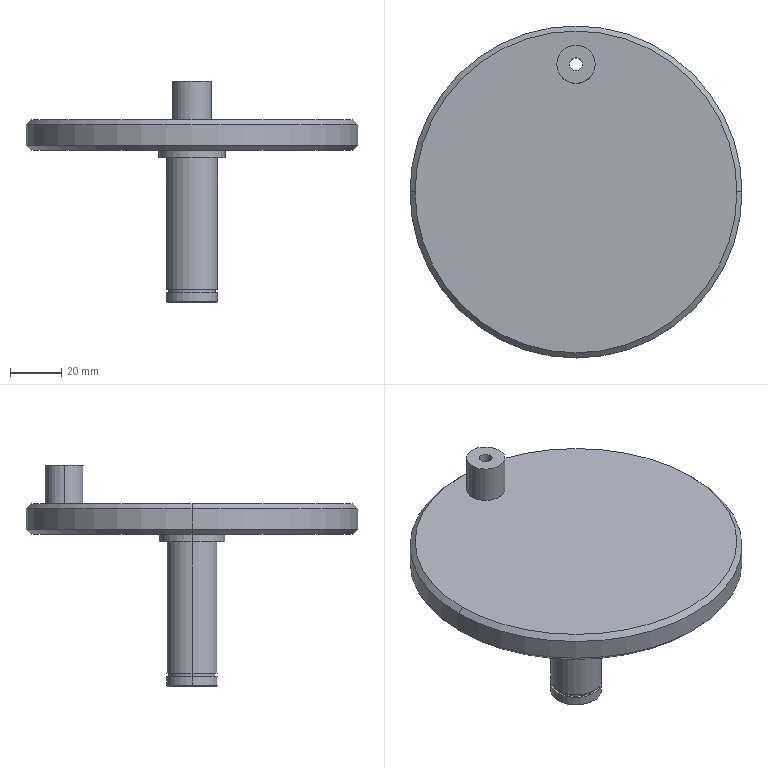Part | SolidWorks | features BaseBody 1 | 1 solid | 27 faces | box 130 x 130 x 86.7 mm | volume 179121 mm3 | cylinder 14 | plane 7 | cone 6 | commonest cylinder face diameters 20 x4 5 x2 15 x2 18.35 x2 26 x2 130 x2
STEP:
#1=CARTESIAN_POINT('',(-9.175,0.,-55.7));
#2=VERTEX_POINT('',#1);
#3=CARTESIAN_POINT('',(9.175,0.,-55.7));
#4=VERTEX_POINT('',#3);
#5=CARTESIAN_POINT('',(0.,0.,-55.7));
#6=DIRECTION('',(0.,0.,-1.));
#7=DIRECTION('',(1.,0.,0.));
#8=AXIS2_PLACEMENT_3D('',#5,#6,#7);
#9=CIRCLE('',#8,9.175);
#10=EDGE_CURVE('',#2,#4,#9,.T.);
#11=ORIENTED_EDGE('',*,*,#10,.F.);
#12=CARTESIAN_POINT('',(-9.175,0.,-54.5));
#13=VERTEX_POINT('',#12);
#14=CARTESIAN_POINT('',(-9.175,0.,-55.1));
#15=DIRECTION('',(0.,0.,1.));
#16=VECTOR('',#15,1000.);
#17=LINE('',#14,#16);
#18=EDGE_CURVE('',#2,#13,#17,.T.);
#19=ORIENTED_EDGE('',*,*,#18,.T.);
#20=CARTESIAN_POINT('',(9.175,0.,-54.5));
#21=VERTEX_POINT('',#20);
#22=CARTESIAN_POINT('',(0.,0.,-54.5));
#23=DIRECTION('',(0.,0.,-1.));
#24=DIRECTION('',(1.,0.,0.));
#25=AXIS2_PLACEMENT_3D('',#22,#23,#24);
#26=CIRCLE('',#25,9.175);
#27=EDGE_CURVE('',#13,#21,#26,.T.);
#28=ORIENTED_EDGE('',*,*,#27,.T.);
#29=CARTESIAN_POINT('',(9.175,0.,-55.1));
#30=DIRECTION('',(0.,0.,1.));
#31=VECTOR('',#30,1000.);
#32=LINE('',#29,#31);
#33=EDGE_CURVE('',#4,#21,#32,.T.);
#34=ORIENTED_EDGE('',*,*,#33,.F.);
#35=EDGE_LOOP('',(#11,#19,#28,#34));
#36=FACE_OUTER_BOUND('',#35,.T.);
#37=CARTESIAN_POINT('',(0.,0.,-55.1));
#38=DIRECTION('',(0.,0.,1.));
#39=DIRECTION('',(1.,0.,0.));
#40=AXIS2_PLACEMENT_3D('',#37,#38,#39);
#41=CYLINDRICAL_SURFACE('',#40,9.175);
#42=ADVANCED_FACE('',(#36),#41,.T.);
#43=CARTESIAN_POINT('',(10.,0.,-54.5));
#44=VERTEX_POINT('',#43);
#45=CARTESIAN_POINT('',(-10.,0.,-54.5));
#46=VERTEX_POINT('',#45);
#47=CARTESIAN_POINT('',(0.,0.,-54.5));
#48=DIRECTION('',(0.,0.,1.));
#49=DIRECTION('',(1.,0.,0.));
#50=AXIS2_PLACEMENT_3D('',#47,#48,#49);
#51=CIRCLE('',#50,10.);
#52=EDGE_CURVE('',#44,#46,#51,.T.);
#53=ORIENTED_EDGE('',*,*,#52,.T.);
#54=CARTESIAN_POINT('',(-10.,0.,-3.));
#55=VERTEX_POINT('',#54);
#56=CARTESIAN_POINT('',(-10.,0.,0.));
#57=DIRECTION('',(0.,0.,1.));
#58=VECTOR('',#57,1000.);
#59=LINE('',#56,#58);
#60=EDGE_CURVE('',#46,#55,#59,.T.);
#61=ORIENTED_EDGE('',*,*,#60,.T.);
#62=CARTESIAN_POINT('',(10.,0.,-3.));
#63=VERTEX_POINT('',#62);
#64=CARTESIAN_POINT('',(0.,0.,-3.));
#65=DIRECTION('',(0.,0.,-1.));
#66=DIRECTION('',(1.,0.,0.));
#67=AXIS2_PLACEMENT_3D('',#64,#65,#66);
#68=CIRCLE('',#67,10.);
#69=EDGE_CURVE('',#55,#63,#68,.T.);
#70=ORIENTED_EDGE('',*,*,#69,.T.);
#71=CARTESIAN_POINT('',(10.,0.,0.));
#72=DIRECTION('',(0.,0.,1.));
#73=VECTOR('',#72,1000.);
#74=LINE('',#71,#73);
#75=EDGE_CURVE('',#44,#63,#74,.T.);
#76=ORIENTED_EDGE('',*,*,#75,.F.);
#77=EDGE_LOOP('',(#53,#61,#70,#76));
#78=FACE_OUTER_BOUND('',#77,.T.);
#79=CARTESIAN_POINT('',(0.,0.,0.));
#80=DIRECTION('',(0.,0.,1.));
#81=DIRECTION('',(1.,0.,0.));
#82=AXIS2_PLACEMENT_3D('',#79,#80,#81);
#83=CYLINDRICAL_SURFACE('',#82,10.);
#84=ADVANCED_FACE('',(#78),#83,.T.);
#85=CARTESIAN_POINT('',(9.5,0.,-59.7));
#86=VERTEX_POINT('',#85);
#87=CARTESIAN_POINT('',(-9.5,0.,-59.7));
#88=VERTEX_POINT('',#87);
#89=CARTESIAN_POINT('',(0.,0.,-59.7));
#90=DIRECTION('',(0.,0.,1.));
#91=DIRECTION('',(1.,0.,0.));
#92=AXIS2_PLACEMENT_3D('',#89,#90,#91);
#93=CIRCLE('',#92,9.5);
#94=EDGE_CURVE('',#86,#88,#93,.T.);
#95=ORIENTED_EDGE('',*,*,#94,.T.);
#96=CARTESIAN_POINT('',(-10.,0.,-59.2));
#97=VERTEX_POINT('',#96);
#98=CARTESIAN_POINT('',(-9.75,0.,-59.45));
#99=DIRECTION('',(-0.7071,0.,0.7071));
#100=VECTOR('',#99,1000.);
#101=LINE('',#98,#100);
#102=EDGE_CURVE('',#88,#97,#101,.T.);
#103=ORIENTED_EDGE('',*,*,#102,.T.);
#104=CARTESIAN_POINT('',(10.,0.,-59.2));
#105=VERTEX_POINT('',#104);
#106=CARTESIAN_POINT('',(0.,0.,-59.2));
#107=DIRECTION('',(0.,0.,-1.));
#108=DIRECTION('',(1.,0.,0.));
#109=AXIS2_PLACEMENT_3D('',#106,#107,#108);
#110=CIRCLE('',#109,10.);
#111=EDGE_CURVE('',#97,#105,#110,.T.);
#112=ORIENTED_EDGE('',*,*,#111,.T.);
#113=CARTESIAN_POINT('',(9.75,0.,-59.45));
#114=DIRECTION('',(0.7071,0.,0.7071));
#115=VECTOR('',#114,1000.);
#116=LINE('',#113,#115);
#117=EDGE_CURVE('',#86,#105,#116,.T.);
#118=ORIENTED_EDGE('',*,*,#117,.F.);
#119=EDGE_LOOP('',(#95,#103,#112,#118));
#120=FACE_OUTER_BOUND('',#119,.T.);
#121=CARTESIAN_POINT('',(0.,0.,-59.45));
#122=DIRECTION('',(0.,0.,1.));
#123=DIRECTION('',(1.,0.,0.));
#124=AXIS2_PLACEMENT_3D('',#121,#122,#123);
#125=CONICAL_SURFACE('',#124,9.75,0.7854);
#126=ADVANCED_FACE('',(#120),#125,.T.);
#127=ORIENTED_EDGE('',*,*,#111,.F.);
#128=CARTESIAN_POINT('',(-10.,0.,-55.7));
#129=VERTEX_POINT('',#128);
#130=CARTESIAN_POINT('',(-10.,0.,0.));
#131=DIRECTION('',(0.,0.,1.));
#132=VECTOR('',#131,1000.);
#133=LINE('',#130,#132);
#134=EDGE_CURVE('',#97,#129,#133,.T.);
#135=ORIENTED_EDGE('',*,*,#134,.T.);
#136=CARTESIAN_POINT('',(10.,0.,-55.7));
#137=VERTEX_POINT('',#136);
#138=CARTESIAN_POINT('',(0.,0.,-55.7));
#139=DIRECTION('',(0.,0.,-1.));
#140=DIRECTION('',(1.,0.,0.));
#141=AXIS2_PLACEMENT_3D('',#138,#139,#140);
#142=CIRCLE('',#141,10.);
#143=EDGE_CURVE('',#129,#137,#142,.T.);
#144=ORIENTED_EDGE('',*,*,#143,.T.);
#145=CARTESIAN_POINT('',(10.,0.,0.));
#146=DIRECTION('',(0.,0.,1.));
#147=VECTOR('',#146,1000.);
#148=LINE('',#145,#147);
#149=EDGE_CURVE('',#105,#137,#148,.T.);
#150=ORIENTED_EDGE('',*,*,#149,.F.);
#151=EDGE_LOOP('',(#127,#135,#144,#150));
#152=FACE_OUTER_BOUND('',#151,.T.);
#153=CARTESIAN_POINT('',(0.,0.,0.));
#154=DIRECTION('',(0.,0.,1.));
#155=DIRECTION('',(1.,0.,0.));
#156=AXIS2_PLACEMENT_3D('',#153,#154,#155);
#157=CYLINDRICAL_SURFACE('',#156,10.);
#158=ADVANCED_FACE('',(#152),#157,.T.);
#159=CARTESIAN_POINT('',(-63.,0.,12.));
#160=VERTEX_POINT('',#159);
#161=CARTESIAN_POINT('',(63.,0.,12.));
#162=VERTEX_POINT('',#161);
#163=CARTESIAN_POINT('',(0.,0.,12.));
#164=DIRECTION('',(0.,0.,-1.));
#165=DIRECTION('',(-1.,0.,0.));
#166=AXIS2_PLACEMENT_3D('',#163,#164,#165);
#167=CIRCLE('',#166,63.);
#168=EDGE_CURVE('',#160,#162,#167,.T.);
#169=ORIENTED_EDGE('',*,*,#168,.T.);
#170=CARTESIAN_POINT('',(65.,0.,10.));
#171=VERTEX_POINT('',#170);
#172=CARTESIAN_POINT('',(64.,0.,11.));
#173=DIRECTION('',(0.7071,0.,-0.7071));
#174=VECTOR('',#173,1000.);
#175=LINE('',#172,#174);
#176=EDGE_CURVE('',#162,#171,#175,.T.);
#177=ORIENTED_EDGE('',*,*,#176,.T.);
#178=CARTESIAN_POINT('',(-65.,0.,10.));
#179=VERTEX_POINT('',#178);
#180=CARTESIAN_POINT('',(0.,0.,10.));
#181=DIRECTION('',(0.,0.,1.));
#182=DIRECTION('',(-1.,0.,0.));
#183=AXIS2_PLACEMENT_3D('',#180,#181,#182);
#184=CIRCLE('',#183,65.);
#185=EDGE_CURVE('',#171,#179,#184,.T.);
#186=ORIENTED_EDGE('',*,*,#185,.T.);
#187=CARTESIAN_POINT('',(-64.,0.,11.));
#188=DIRECTION('',(-0.7071,0.,-0.7071));
#189=VECTOR('',#188,1000.);
#190=LINE('',#187,#189);
#191=EDGE_CURVE('',#160,#179,#190,.T.);
#192=ORIENTED_EDGE('',*,*,#191,.F.);
#193=EDGE_LOOP('',(#169,#177,#186,#192));
#194=FACE_OUTER_BOUND('',#193,.T.);
#195=CARTESIAN_POINT('',(0.,0.,11.));
#196=DIRECTION('',(0.,0.,-1.));
#197=DIRECTION('',(-1.,0.,0.));
#198=AXIS2_PLACEMENT_3D('',#195,#196,#197);
#199=CONICAL_SURFACE('',#198,64.,0.7854);
#200=ADVANCED_FACE('',(#194),#199,.T.);
#201=ORIENTED_EDGE('',*,*,#185,.F.);
#202=CARTESIAN_POINT('',(65.,0.,2.));
#203=VERTEX_POINT('',#202);
#204=CARTESIAN_POINT('',(65.,0.,0.));
#205=DIRECTION('',(0.,0.,-1.));
#206=VECTOR('',#205,1000.);
#207=LINE('',#204,#206);
#208=EDGE_CURVE('',#171,#203,#207,.T.);
#209=ORIENTED_EDGE('',*,*,#208,.T.);
#210=CARTESIAN_POINT('',(-65.,0.,2.));
#211=VERTEX_POINT('',#210);
#212=CARTESIAN_POINT('',(0.,0.,2.));
#213=DIRECTION('',(0.,0.,-1.));
#214=DIRECTION('',(-1.,0.,0.));
#215=AXIS2_PLACEMENT_3D('',#212,#213,#214);
#216=CIRCLE('',#215,65.);
#217=EDGE_CURVE('',#211,#203,#216,.T.);
#218=ORIENTED_EDGE('',*,*,#217,.F.);
#219=CARTESIAN_POINT('',(-65.,0.,0.));
#220=DIRECTION('',(0.,0.,-1.));
#221=VECTOR('',#220,1000.);
#222=LINE('',#219,#221);
#223=EDGE_CURVE('',#179,#211,#222,.T.);
#224=ORIENTED_EDGE('',*,*,#223,.F.);
#225=EDGE_LOOP('',(#201,#209,#218,#224));
#226=FACE_OUTER_BOUND('',#225,.T.);
#227=CARTESIAN_POINT('',(0.,0.,0.));
#228=DIRECTION('',(0.,0.,-1.));
#229=DIRECTION('',(-1.,0.,0.));
#230=AXIS2_PLACEMENT_3D('',#227,#228,#229);
#231=CYLINDRICAL_SURFACE('',#230,65.);
#232=ADVANCED_FACE('',(#226),#231,.T.);
#233=CARTESIAN_POINT('',(-63.,0.,0.));
#234=VERTEX_POINT('',#233);
#235=CARTESIAN_POINT('',(63.,0.,0.));
#236=VERTEX_POINT('',#235);
#237=CARTESIAN_POINT('',(0.,0.,0.));
#238=DIRECTION('',(0.,0.,1.));
#239=DIRECTION('',(-1.,0.,0.));
#240=AXIS2_PLACEMENT_3D('',#237,#238,#239);
#241=CIRCLE('',#240,63.);
#242=EDGE_CURVE('',#234,#236,#241,.T.);
#243=ORIENTED_EDGE('',*,*,#242,.T.);
#244=CARTESIAN_POINT('',(64.,0.,1.));
#245=DIRECTION('',(0.7071,0.,0.7071));
#246=VECTOR('',#245,1000.);
#247=LINE('',#244,#246);
#248=EDGE_CURVE('',#236,#203,#247,.T.);
#249=ORIENTED_EDGE('',*,*,#248,.T.);
#250=CARTESIAN_POINT('',(0.,0.,2.));
#251=DIRECTION('',(0.,0.,-1.));
#252=DIRECTION('',(-1.,0.,0.));
#253=AXIS2_PLACEMENT_3D('',#250,#251,#252);
#254=CIRCLE('',#253,65.);
#255=EDGE_CURVE('',#203,#211,#254,.T.);
#256=ORIENTED_EDGE('',*,*,#255,.T.);
#257=CARTESIAN_POINT('',(-64.,0.,1.));
#258=DIRECTION('',(-0.7071,0.,0.7071));
#259=VECTOR('',#258,1000.);
#260=LINE('',#257,#259);
#261=EDGE_CURVE('',#234,#211,#260,.T.);
#262=ORIENTED_EDGE('',*,*,#261,.F.);
#263=EDGE_LOOP('',(#243,#249,#256,#262));
#264=FACE_OUTER_BOUND('',#263,.T.);
#265=CARTESIAN_POINT('',(0.,0.,1.));
#266=DIRECTION('',(0.,0.,1.));
#267=DIRECTION('',(-1.,0.,0.));
#268=AXIS2_PLACEMENT_3D('',#265,#266,#267);
#269=CONICAL_SURFACE('',#268,64.,0.7854);
#270=ADVANCED_FACE('',(#264),#269,.T.);
#271=CARTESIAN_POINT('',(-13.,0.,-3.));
#272=VERTEX_POINT('',#271);
#273=CARTESIAN_POINT('',(13.,0.,-3.));
#274=VERTEX_POINT('',#273);
#275=CARTESIAN_POINT('',(0.,0.,-3.));
#276=DIRECTION('',(0.,0.,-1.));
#277=DIRECTION('',(1.,0.,0.));
#278=AXIS2_PLACEMENT_3D('',#275,#276,#277);
#279=CIRCLE('',#278,13.);
#280=EDGE_CURVE('',#272,#274,#279,.T.);
#281=ORIENTED_EDGE('',*,*,#280,.F.);
#282=CARTESIAN_POINT('',(-13.,0.,0.));
#283=VERTEX_POINT('',#282);
#284=CARTESIAN_POINT('',(-13.,0.,0.));
#285=DIRECTION('',(0.,0.,1.));
#286=VECTOR('',#285,1000.);
#287=LINE('',#284,#286);
#288=EDGE_CURVE('',#272,#283,#287,.T.);
#289=ORIENTED_EDGE('',*,*,#288,.T.);
#290=CARTESIAN_POINT('',(13.,0.,0.));
#291=VERTEX_POINT('',#290);
#292=CARTESIAN_POINT('',(0.,0.,0.));
#293=DIRECTION('',(0.,0.,1.));
#294=DIRECTION('',(1.,0.,0.));
#295=AXIS2_PLACEMENT_3D('',#292,#293,#294);
#296=CIRCLE('',#295,13.);
#297=EDGE_CURVE('',#291,#283,#296,.T.);
#298=ORIENTED_EDGE('',*,*,#297,.F.);
#299=CARTESIAN_POINT('',(13.,0.,0.));
#300=DIRECTION('',(0.,0.,1.));
#301=VECTOR('',#300,1000.);
#302=LINE('',#299,#301);
#303=EDGE_CURVE('',#274,#291,#302,.T.);
#304=ORIENTED_EDGE('',*,*,#303,.F.);
#305=EDGE_LOOP('',(#281,#289,#298,#304));
#306=FACE_OUTER_BOUND('',#305,.T.);
#307=CARTESIAN_POINT('',(0.,0.,0.));
#308=DIRECTION('',(0.,0.,1.));
#309=DIRECTION('',(1.,0.,0.));
#310=AXIS2_PLACEMENT_3D('',#307,#308,#309);
#311=CYLINDRICAL_SURFACE('',#310,13.);
#312=ADVANCED_FACE('',(#306),#311,.T.);
#313=CARTESIAN_POINT('',(2.5,50.,0.));
#314=VERTEX_POINT('',#313);
#315=CARTESIAN_POINT('',(-2.5,50.,0.));
#316=VERTEX_POINT('',#315);
#317=CARTESIAN_POINT('',(0.,50.,0.));
#318=DIRECTION('',(0.,0.,1.));
#319=DIRECTION('',(-1.,0.,0.));
#320=AXIS2_PLACEMENT_3D('',#317,#318,#319);
#321=CIRCLE('',#320,2.5);
#322=EDGE_CURVE('',#314,#316,#321,.T.);
#323=ORIENTED_EDGE('',*,*,#322,.F.);
#324=CARTESIAN_POINT('',(2.5,50.,27.));
#325=VERTEX_POINT('',#324);
#326=CARTESIAN_POINT('',(2.5,50.,27.));
#327=DIRECTION('',(0.,0.,1.));
#328=VECTOR('',#327,1000.);
#329=LINE('',#326,#328);
#330=EDGE_CURVE('',#314,#325,#329,.T.);
#331=ORIENTED_EDGE('',*,*,#330,.T.);
#332=CARTESIAN_POINT('',(-2.5,50.,27.));
#333=VERTEX_POINT('',#332);
#334=CARTESIAN_POINT('',(0.,50.,27.));
#335=DIRECTION('',(0.,0.,-1.));
#336=DIRECTION('',(-1.,0.,0.));
#337=AXIS2_PLACEMENT_3D('',#334,#335,#336);
#338=CIRCLE('',#337,2.5);
#339=EDGE_CURVE('',#333,#325,#338,.T.);
#340=ORIENTED_EDGE('',*,*,#339,.F.);
#341=CARTESIAN_POINT('',(-2.5,50.,27.));
#342=DIRECTION('',(0.,0.,1.));
#343=VECTOR('',#342,1000.);
#344=LINE('',#341,#343);
#345=EDGE_CURVE('',#316,#333,#344,.T.);
#346=ORIENTED_EDGE('',*,*,#345,.F.);
#347=EDGE_LOOP('',(#323,#331,#340,#346));
#348=FACE_OUTER_BOUND('',#347,.T.);
#349=CARTESIAN_POINT('',(0.,50.,27.));
#350=DIRECTION('',(0.,0.,1.));
#351=DIRECTION('',(-1.,0.,0.));
#352=AXIS2_PLACEMENT_3D('',#349,#350,#351);
#353=CYLINDRICAL_SURFACE('',#352,2.5);
#354=ADVANCED_FACE('',(#348),#353,.F.);
#355=CARTESIAN_POINT('',(7.5,50.,27.));
#356=VERTEX_POINT('',#355);
#357=CARTESIAN_POINT('',(-7.5,50.,27.));
#358=VERTEX_POINT('',#357);
#359=CARTESIAN_POINT('',(0.,50.,27.));
#360=DIRECTION('',(0.,0.,1.));
#361=DIRECTION('',(-1.,0.,0.));
#362=AXIS2_PLACEMENT_3D('',#359,#360,#361);
#363=CIRCLE('',#362,7.5);
#364=EDGE_CURVE('',#356,#358,#363,.T.);
#365=ORIENTED_EDGE('',*,*,#364,.F.);
#366=CARTESIAN_POINT('',(7.5,50.,12.));
#367=VERTEX_POINT('',#366);
#368=CARTESIAN_POINT('',(7.5,50.,12.));
#369=DIRECTION('',(0.,0.,-1.));
#370=VECTOR('',#369,1000.);
#371=LINE('',#368,#370);
#372=EDGE_CURVE('',#356,#367,#371,.T.);
#373=ORIENTED_EDGE('',*,*,#372,.T.);
#374=CARTESIAN_POINT('',(-7.5,50.,12.));
#375=VERTEX_POINT('',#374);
#376=CARTESIAN_POINT('',(0.,50.,12.));
#377=DIRECTION('',(0.,0.,-1.));
#378=DIRECTION('',(-1.,0.,0.));
#379=AXIS2_PLACEMENT_3D('',#376,#377,#378);
#380=CIRCLE('',#379,7.5);
#381=EDGE_CURVE('',#375,#367,#380,.T.);
#382=ORIENTED_EDGE('',*,*,#381,.F.);
#383=CARTESIAN_POINT('',(-7.5,50.,12.));
#384=DIRECTION('',(0.,0.,-1.));
#385=VECTOR('',#384,1000.);
#386=LINE('',#383,#385);
#387=EDGE_CURVE('',#358,#375,#386,.T.);
#388=ORIENTED_EDGE('',*,*,#387,.F.);
#389=EDGE_LOOP('',(#365,#373,#382,#388));
#390=FACE_OUTER_BOUND('',#389,.T.);
#391=CARTESIAN_POINT('',(0.,50.,12.));
#392=DIRECTION('',(0.,0.,-1.));
#393=DIRECTION('',(-1.,0.,0.));
#394=AXIS2_PLACEMENT_3D('',#391,#392,#393);
#395=CYLINDRICAL_SURFACE('',#394,7.5);
#396=ADVANCED_FACE('',(#390),#395,.T.);
#397=CARTESIAN_POINT('',(0.,0.,-55.7));
#398=DIRECTION('',(0.,0.,-1.));
#399=DIRECTION('',(1.,0.,0.));
#400=AXIS2_PLACEMENT_3D('',#397,#398,#399);
#401=CIRCLE('',#400,9.175);
#402=EDGE_CURVE('',#4,#2,#401,.T.);
#403=ORIENTED_EDGE('',*,*,#402,.T.);
#404=ORIENTED_EDGE('',*,*,#10,.T.);
#405=EDGE_LOOP('',(#403,#404));
#406=FACE_BOUND('',#405,.T.);
#407=CARTESIAN_POINT('',(0.,0.,-55.7));
#408=DIRECTION('',(0.,0.,-1.));
#409=DIRECTION('',(1.,0.,0.));
#410=AXIS2_PLACEMENT_3D('',#407,#408,#409);
#411=CIRCLE('',#410,10.);
#412=EDGE_CURVE('',#137,#129,#411,.T.);
#413=ORIENTED_EDGE('',*,*,#412,.F.);
#414=ORIENTED_EDGE('',*,*,#143,.F.);
#415=EDGE_LOOP('',(#413,#414));
#416=FACE_OUTER_BOUND('',#415,.T.);
#417=CARTESIAN_POINT('',(9.175,0.,-55.7));
#418=DIRECTION('',(0.,0.,-1.));
#419=DIRECTION('',(0.,-1.,0.));
#420=AXIS2_PLACEMENT_3D('',#417,#418,#419);
#421=PLANE('',#420);
#422=ADVANCED_FACE('',(#406,#416),#421,.F.);
#423=CARTESIAN_POINT('',(0.,0.,-54.5));
#424=DIRECTION('',(0.,0.,-1.));
#425=DIRECTION('',(1.,0.,0.));
#426=AXIS2_PLACEMENT_3D('',#423,#424,#425);
#427=CIRCLE('',#426,9.175);
#428=EDGE_CURVE('',#21,#13,#427,.T.);
#429=ORIENTED_EDGE('',*,*,#428,.F.);
#430=ORIENTED_EDGE('',*,*,#27,.F.);
#431=EDGE_LOOP('',(#429,#430));
#432=FACE_BOUND('',#431,.T.);
#433=ORIENTED_EDGE('',*,*,#52,.F.);
#434=CARTESIAN_POINT('',(0.,0.,-54.5));
#435=DIRECTION('',(0.,0.,1.));
#436=DIRECTION('',(1.,0.,0.));
#437=AXIS2_PLACEMENT_3D('',#434,#435,#436);
#438=CIRCLE('',#437,10.);
#439=EDGE_CURVE('',#46,#44,#438,.T.);
#440=ORIENTED_EDGE('',*,*,#439,.F.);
#441=EDGE_LOOP('',(#433,#440));
#442=FACE_OUTER_BOUND('',#441,.T.);
#443=CARTESIAN_POINT('',(18.451,0.,-54.5));
#444=DIRECTION('',(0.,0.,1.));
#445=DIRECTION('',(1.,0.,0.));
#446=AXIS2_PLACEMENT_3D('',#443,#444,#445);
#447=PLANE('',#446);
#448=ADVANCED_FACE('',(#432,#442),#447,.F.);
#449=ORIENTED_EDGE('',*,*,#94,.F.);
#450=CARTESIAN_POINT('',(0.,0.,-59.7));
#451=DIRECTION('',(0.,0.,1.));
#452=DIRECTION('',(1.,0.,0.));
#453=AXIS2_PLACEMENT_3D('',#450,#451,#452);
#454=CIRCLE('',#453,9.5);
#455=EDGE_CURVE('',#88,#86,#454,.T.);
#456=ORIENTED_EDGE('',*,*,#455,.F.);
#457=EDGE_LOOP('',(#449,#456));
#458=FACE_OUTER_BOUND('',#457,.T.);
#459=CARTESIAN_POINT('',(0.,0.,-59.7));
#460=DIRECTION('',(0.,0.,1.));
#461=DIRECTION('',(1.,0.,0.));
#462=AXIS2_PLACEMENT_3D('',#459,#460,#461);
#463=PLANE('',#462);
#464=ADVANCED_FACE('',(#458),#463,.F.);
#465=ORIENTED_EDGE('',*,*,#381,.T.);
#466=CARTESIAN_POINT('',(0.,50.,12.));
#467=DIRECTION('',(0.,0.,-1.));
#468=DIRECTION('',(-1.,0.,0.));
#469=AXIS2_PLACEMENT_3D('',#466,#467,#468);
#470=CIRCLE('',#469,7.5);
#471=EDGE_CURVE('',#367,#375,#470,.T.);
#472=ORIENTED_EDGE('',*,*,#471,.T.);
#473=EDGE_LOOP('',(#465,#472));
#474=FACE_BOUND('',#473,.T.);
#475=ORIENTED_EDGE('',*,*,#168,.F.);
#476=CARTESIAN_POINT('',(0.,0.,12.));
#477=DIRECTION('',(0.,0.,-1.));
#478=DIRECTION('',(-1.,0.,0.));
#479=AXIS2_PLACEMENT_3D('',#476,#477,#478);
#480=CIRCLE('',#479,63.);
#481=EDGE_CURVE('',#162,#160,#480,.T.);
#482=ORIENTED_EDGE('',*,*,#481,.F.);
#483=EDGE_LOOP('',(#475,#482));
#484=FACE_OUTER_BOUND('',#483,.T.);
#485=CARTESIAN_POINT('',(0.,0.,12.));
#486=DIRECTION('',(0.,0.,1.));
#487=DIRECTION('',(1.,0.,0.));
#488=AXIS2_PLACEMENT_3D('',#485,#486,#487);
#489=PLANE('',#488);
#490=ADVANCED_FACE('',(#474,#484),#489,.T.);
#491=CARTESIAN_POINT('',(0.,50.,0.));
#492=DIRECTION('',(0.,0.,1.));
#493=DIRECTION('',(-1.,0.,0.));
#494=AXIS2_PLACEMENT_3D('',#491,#492,#493);
#495=CIRCLE('',#494,2.5);
#496=EDGE_CURVE('',#316,#314,#495,.T.);
#497=ORIENTED_EDGE('',*,*,#496,.T.);
#498=ORIENTED_EDGE('',*,*,#322,.T.);
#499=EDGE_LOOP('',(#497,#498));
#500=FACE_BOUND('',#499,.T.);
#501=ORIENTED_EDGE('',*,*,#297,.T.);
#502=CARTESIAN_POINT('',(0.,0.,0.));
#503=DIRECTION('',(0.,0.,1.));
#504=DIRECTION('',(1.,0.,0.));
#505=AXIS2_PLACEMENT_3D('',#502,#503,#504);
#506=CIRCLE('',#505,13.);
#507=EDGE_CURVE('',#283,#291,#506,.T.);
#508=ORIENTED_EDGE('',*,*,#507,.T.);
#509=EDGE_LOOP('',(#501,#508));
#510=FACE_BOUND('',#509,.T.);
#511=ORIENTED_EDGE('',*,*,#242,.F.);
#512=CARTESIAN_POINT('',(0.,0.,0.));
#513=DIRECTION('',(0.,0.,1.));
#514=DIRECTION('',(-1.,0.,0.));
#515=AXIS2_PLACEMENT_3D('',#512,#513,#514);
#516=CIRCLE('',#515,63.);
#517=EDGE_CURVE('',#236,#234,#516,.T.);
#518=ORIENTED_EDGE('',*,*,#517,.F.);
#519=EDGE_LOOP('',(#511,#518));
#520=FACE_OUTER_BOUND('',#519,.T.);
#521=CARTESIAN_POINT('',(0.,0.,0.));
#522=DIRECTION('',(0.,0.,1.));
#523=DIRECTION('',(1.,0.,0.));
#524=AXIS2_PLACEMENT_3D('',#521,#522,#523);
#525=PLANE('',#524);
#526=ADVANCED_FACE('',(#500,#510,#520),#525,.F.);
#527=CARTESIAN_POINT('',(0.,0.,-3.));
#528=DIRECTION('',(0.,0.,-1.));
#529=DIRECTION('',(1.,0.,0.));
#530=AXIS2_PLACEMENT_3D('',#527,#528,#529);
#531=CIRCLE('',#530,10.);
#532=EDGE_CURVE('',#63,#55,#531,.T.);
#533=ORIENTED_EDGE('',*,*,#532,.F.);
#534=ORIENTED_EDGE('',*,*,#69,.F.);
#535=EDGE_LOOP('',(#533,#534));
#536=FACE_BOUND('',#535,.T.);
#537=CARTESIAN_POINT('',(0.,0.,-3.));
#538=DIRECTION('',(0.,0.,-1.));
#539=DIRECTION('',(1.,0.,0.));
#540=AXIS2_PLACEMENT_3D('',#537,#538,#539);
#541=CIRCLE('',#540,13.);
#542=EDGE_CURVE('',#274,#272,#541,.T.);
#543=ORIENTED_EDGE('',*,*,#542,.T.);
#544=ORIENTED_EDGE('',*,*,#280,.T.);
#545=EDGE_LOOP('',(#543,#544));
#546=FACE_OUTER_BOUND('',#545,.T.);
#547=CARTESIAN_POINT('',(0.,0.,-3.));
#548=DIRECTION('',(0.,0.,1.));
#549=DIRECTION('',(1.,0.,0.));
#550=AXIS2_PLACEMENT_3D('',#547,#548,#549);
#551=PLANE('',#550);
#552=ADVANCED_FACE('',(#536,#546),#551,.F.);
#553=ORIENTED_EDGE('',*,*,#339,.T.);
#554=CARTESIAN_POINT('',(0.,50.,27.));
#555=DIRECTION('',(0.,0.,-1.));
#556=DIRECTION('',(-1.,0.,0.));
#557=AXIS2_PLACEMENT_3D('',#554,#555,#556);
#558=CIRCLE('',#557,2.5);
#559=EDGE_CURVE('',#325,#333,#558,.T.);
#560=ORIENTED_EDGE('',*,*,#559,.T.);
#561=EDGE_LOOP('',(#553,#560));
#562=FACE_BOUND('',#561,.T.);
#563=CARTESIAN_POINT('',(0.,50.,27.));
#564=DIRECTION('',(0.,0.,1.));
#565=DIRECTION('',(-1.,0.,0.));
#566=AXIS2_PLACEMENT_3D('',#563,#564,#565);
#567=CIRCLE('',#566,7.5);
#568=EDGE_CURVE('',#358,#356,#567,.T.);
#569=ORIENTED_EDGE('',*,*,#568,.T.);
#570=ORIENTED_EDGE('',*,*,#364,.T.);
#571=EDGE_LOOP('',(#569,#570));
#572=FACE_OUTER_BOUND('',#571,.T.);
#573=CARTESIAN_POINT('',(0.,50.,27.));
#574=DIRECTION('',(0.,0.,1.));
#575=DIRECTION('',(1.,0.,0.));
#576=AXIS2_PLACEMENT_3D('',#573,#574,#575);
#577=PLANE('',#576);
#578=ADVANCED_FACE('',(#562,#572),#577,.T.);
#579=ORIENTED_EDGE('',*,*,#372,.F.);
#580=ORIENTED_EDGE('',*,*,#568,.F.);
#581=ORIENTED_EDGE('',*,*,#387,.T.);
#582=ORIENTED_EDGE('',*,*,#471,.F.);
#583=EDGE_LOOP('',(#579,#580,#581,#582));
#584=FACE_OUTER_BOUND('',#583,.T.);
#585=CARTESIAN_POINT('',(0.,50.,12.));
#586=DIRECTION('',(0.,0.,-1.));
#587=DIRECTION('',(-1.,0.,0.));
#588=AXIS2_PLACEMENT_3D('',#585,#586,#587);
#589=CYLINDRICAL_SURFACE('',#588,7.5);
#590=ADVANCED_FACE('',(#584),#589,.T.);
#591=ORIENTED_EDGE('',*,*,#330,.F.);
#592=ORIENTED_EDGE('',*,*,#496,.F.);
#593=ORIENTED_EDGE('',*,*,#345,.T.);
#594=ORIENTED_EDGE('',*,*,#559,.F.);
#595=EDGE_LOOP('',(#591,#592,#593,#594));
#596=FACE_OUTER_BOUND('',#595,.T.);
#597=CARTESIAN_POINT('',(0.,50.,27.));
#598=DIRECTION('',(0.,0.,1.));
#599=DIRECTION('',(-1.,0.,0.));
#600=AXIS2_PLACEMENT_3D('',#597,#598,#599);
#601=CYLINDRICAL_SURFACE('',#600,2.5);
#602=ADVANCED_FACE('',(#596),#601,.F.);
#603=ORIENTED_EDGE('',*,*,#288,.F.);
#604=ORIENTED_EDGE('',*,*,#542,.F.);
#605=ORIENTED_EDGE('',*,*,#303,.T.);
#606=ORIENTED_EDGE('',*,*,#507,.F.);
#607=EDGE_LOOP('',(#603,#604,#605,#606));
#608=FACE_OUTER_BOUND('',#607,.T.);
#609=CARTESIAN_POINT('',(0.,0.,0.));
#610=DIRECTION('',(0.,0.,1.));
#611=DIRECTION('',(1.,0.,0.));
#612=AXIS2_PLACEMENT_3D('',#609,#610,#611);
#613=CYLINDRICAL_SURFACE('',#612,13.);
#614=ADVANCED_FACE('',(#608),#613,.T.);
#615=ORIENTED_EDGE('',*,*,#248,.F.);
#616=ORIENTED_EDGE('',*,*,#517,.T.);
#617=ORIENTED_EDGE('',*,*,#261,.T.);
#618=ORIENTED_EDGE('',*,*,#217,.T.);
#619=EDGE_LOOP('',(#615,#616,#617,#618));
#620=FACE_OUTER_BOUND('',#619,.T.);
#621=CARTESIAN_POINT('',(0.,0.,1.));
#622=DIRECTION('',(0.,0.,1.));
#623=DIRECTION('',(-1.,0.,0.));
#624=AXIS2_PLACEMENT_3D('',#621,#622,#623);
#625=CONICAL_SURFACE('',#624,64.,0.7854);
#626=ADVANCED_FACE('',(#620),#625,.T.);
#627=ORIENTED_EDGE('',*,*,#208,.F.);
#628=CARTESIAN_POINT('',(0.,0.,10.));
#629=DIRECTION('',(0.,0.,1.));
#630=DIRECTION('',(-1.,0.,0.));
#631=AXIS2_PLACEMENT_3D('',#628,#629,#630);
#632=CIRCLE('',#631,65.);
#633=EDGE_CURVE('',#179,#171,#632,.T.);
#634=ORIENTED_EDGE('',*,*,#633,.F.);
#635=ORIENTED_EDGE('',*,*,#223,.T.);
#636=ORIENTED_EDGE('',*,*,#255,.F.);
#637=EDGE_LOOP('',(#627,#634,#635,#636));
#638=FACE_OUTER_BOUND('',#637,.T.);
#639=CARTESIAN_POINT('',(0.,0.,0.));
#640=DIRECTION('',(0.,0.,-1.));
#641=DIRECTION('',(-1.,0.,0.));
#642=AXIS2_PLACEMENT_3D('',#639,#640,#641);
#643=CYLINDRICAL_SURFACE('',#642,65.);
#644=ADVANCED_FACE('',(#638),#643,.T.);
#645=ORIENTED_EDGE('',*,*,#176,.F.);
#646=ORIENTED_EDGE('',*,*,#481,.T.);
#647=ORIENTED_EDGE('',*,*,#191,.T.);
#648=ORIENTED_EDGE('',*,*,#633,.T.);
#649=EDGE_LOOP('',(#645,#646,#647,#648));
#650=FACE_OUTER_BOUND('',#649,.T.);
#651=CARTESIAN_POINT('',(0.,0.,11.));
#652=DIRECTION('',(0.,0.,-1.));
#653=DIRECTION('',(-1.,0.,0.));
#654=AXIS2_PLACEMENT_3D('',#651,#652,#653);
#655=CONICAL_SURFACE('',#654,64.,0.7854);
#656=ADVANCED_FACE('',(#650),#655,.T.);
#657=ORIENTED_EDGE('',*,*,#134,.F.);
#658=CARTESIAN_POINT('',(0.,0.,-59.2));
#659=DIRECTION('',(0.,0.,-1.));
#660=DIRECTION('',(1.,0.,0.));
#661=AXIS2_PLACEMENT_3D('',#658,#659,#660);
#662=CIRCLE('',#661,10.);
#663=EDGE_CURVE('',#105,#97,#662,.T.);
#664=ORIENTED_EDGE('',*,*,#663,.F.);
#665=ORIENTED_EDGE('',*,*,#149,.T.);
#666=ORIENTED_EDGE('',*,*,#412,.T.);
#667=EDGE_LOOP('',(#657,#664,#665,#666));
#668=FACE_OUTER_BOUND('',#667,.T.);
#669=CARTESIAN_POINT('',(0.,0.,0.));
#670=DIRECTION('',(0.,0.,1.));
#671=DIRECTION('',(1.,0.,0.));
#672=AXIS2_PLACEMENT_3D('',#669,#670,#671);
#673=CYLINDRICAL_SURFACE('',#672,10.);
#674=ADVANCED_FACE('',(#668),#673,.T.);
#675=ORIENTED_EDGE('',*,*,#102,.F.);
#676=ORIENTED_EDGE('',*,*,#455,.T.);
#677=ORIENTED_EDGE('',*,*,#117,.T.);
#678=ORIENTED_EDGE('',*,*,#663,.T.);
#679=EDGE_LOOP('',(#675,#676,#677,#678));
#680=FACE_OUTER_BOUND('',#679,.T.);
#681=CARTESIAN_POINT('',(0.,0.,-59.45));
#682=DIRECTION('',(0.,0.,1.));
#683=DIRECTION('',(1.,0.,0.));
#684=AXIS2_PLACEMENT_3D('',#681,#682,#683);
#685=CONICAL_SURFACE('',#684,9.75,0.7854);
#686=ADVANCED_FACE('',(#680),#685,.T.);
#687=ORIENTED_EDGE('',*,*,#60,.F.);
#688=ORIENTED_EDGE('',*,*,#439,.T.);
#689=ORIENTED_EDGE('',*,*,#75,.T.);
#690=ORIENTED_EDGE('',*,*,#532,.T.);
#691=EDGE_LOOP('',(#687,#688,#689,#690));
#692=FACE_OUTER_BOUND('',#691,.T.);
#693=CARTESIAN_POINT('',(0.,0.,0.));
#694=DIRECTION('',(0.,0.,1.));
#695=DIRECTION('',(1.,0.,0.));
#696=AXIS2_PLACEMENT_3D('',#693,#694,#695);
#697=CYLINDRICAL_SURFACE('',#696,10.);
#698=ADVANCED_FACE('',(#692),#697,.T.);
#699=ORIENTED_EDGE('',*,*,#18,.F.);
#700=ORIENTED_EDGE('',*,*,#402,.F.);
#701=ORIENTED_EDGE('',*,*,#33,.T.);
#702=ORIENTED_EDGE('',*,*,#428,.T.);
#703=EDGE_LOOP('',(#699,#700,#701,#702));
#704=FACE_OUTER_BOUND('',#703,.T.);
#705=CARTESIAN_POINT('',(0.,0.,-55.1));
#706=DIRECTION('',(0.,0.,1.));
#707=DIRECTION('',(1.,0.,0.));
#708=AXIS2_PLACEMENT_3D('',#705,#706,#707);
#709=CYLINDRICAL_SURFACE('',#708,9.175);
#710=ADVANCED_FACE('',(#704),#709,.T.);
#711=CLOSED_SHELL('',(#42,#84,#126,#158,#200,#232,#270,#312,#354,#396,#422,#448,#464,#490,#526,#552,#578,#590,#602,#614,#626,#644,#656,#674,#686,#698,#710));
#712=MANIFOLD_SOLID_BREP('',#711);
#713=CARTESIAN_POINT('',(0.,0.,0.));
#714=DIRECTION('',(0.,0.,1.));
#715=DIRECTION('',(1.,0.,0.));
#716=AXIS2_PLACEMENT_3D('',#713,#714,#715);
#717=(LENGTH_UNIT()NAMED_UNIT(*)SI_UNIT(.MILLI.,.METRE.));
#718=UNCERTAINTY_MEASURE_WITH_UNIT(LENGTH_MEASURE(0.00001),#717,'','');
#719=(NAMED_UNIT(*)PLANE_ANGLE_UNIT()SI_UNIT($,.RADIAN.));
#720=(NAMED_UNIT(*)SI_UNIT($,.STERADIAN.)SOLID_ANGLE_UNIT());
#721=(GEOMETRIC_REPRESENTATION_CONTEXT(3)GLOBAL_UNCERTAINTY_ASSIGNED_CONTEXT((#718))GLOBAL_UNIT_ASSIGNED_CONTEXT((#717,#719,#720))REPRESENTATION_CONTEXT('',''));
#722=ADVANCED_BREP_SHAPE_REPRESENTATION('',(#712,#716),#721);